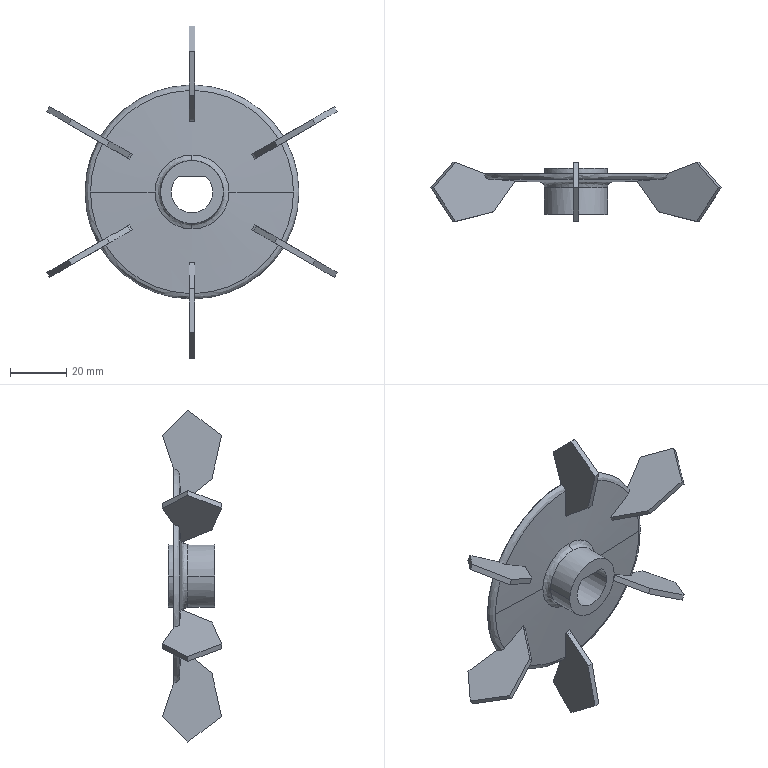Part | SolidWorks | features BaseBody 1 | 1 solid | 98 faces | box 103.191 x 21 x 118 mm | volume 16917 mm3 | plane 63 | spline 16 | cylinder 13 | cone 6 | commonest cylinder face diameters 6 x6 22.4 x4 14.8 x3